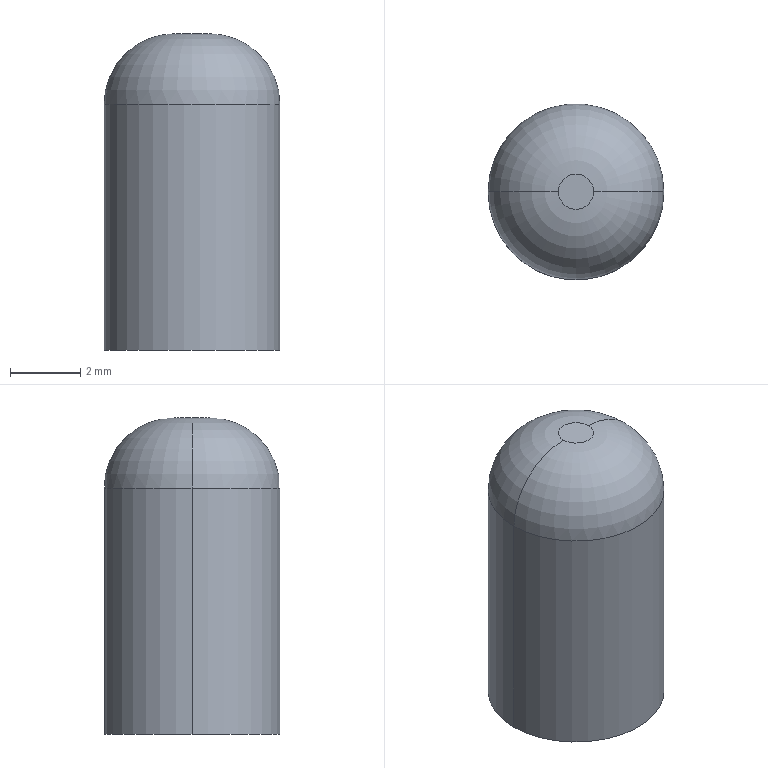Part | SolidWorks | features BaseBody 1 | 1 solid | 6 faces | box 5 x 5 x 9 mm | volume 165.64 mm3 | cylinder 2 | torus 2 | plane 2 | commonest cylinder face diameters 5 x2
STEP:
#1=CARTESIAN_POINT('',(6.125,1.871,0.));
#2=VERTEX_POINT('',#1);
#3=CARTESIAN_POINT('',(1.125,1.871,0.));
#4=VERTEX_POINT('',#3);
#5=CARTESIAN_POINT('',(3.625,1.871,0.));
#6=DIRECTION('',(0.,0.,1.));
#7=DIRECTION('',(1.,0.,0.));
#8=AXIS2_PLACEMENT_3D('',#5,#6,#7);
#9=CIRCLE('',#8,2.5);
#10=EDGE_CURVE('',#2,#4,#9,.T.);
#11=ORIENTED_EDGE('',*,*,#10,.T.);
#12=CARTESIAN_POINT('',(1.125,1.871,7.));
#13=VERTEX_POINT('',#12);
#14=CARTESIAN_POINT('',(1.125,1.871,0.));
#15=DIRECTION('',(0.,0.,1.));
#16=VECTOR('',#15,1000.);
#17=LINE('',#14,#16);
#18=EDGE_CURVE('',#4,#13,#17,.T.);
#19=ORIENTED_EDGE('',*,*,#18,.T.);
#20=CARTESIAN_POINT('',(6.125,1.871,7.));
#21=VERTEX_POINT('',#20);
#22=CARTESIAN_POINT('',(3.625,1.871,7.));
#23=DIRECTION('',(0.,0.,-1.));
#24=DIRECTION('',(1.,0.,0.));
#25=AXIS2_PLACEMENT_3D('',#22,#23,#24);
#26=CIRCLE('',#25,2.5);
#27=EDGE_CURVE('',#13,#21,#26,.T.);
#28=ORIENTED_EDGE('',*,*,#27,.T.);
#29=CARTESIAN_POINT('',(6.125,1.871,0.));
#30=DIRECTION('',(0.,0.,1.));
#31=VECTOR('',#30,1000.);
#32=LINE('',#29,#31);
#33=EDGE_CURVE('',#2,#21,#32,.T.);
#34=ORIENTED_EDGE('',*,*,#33,.F.);
#35=EDGE_LOOP('',(#11,#19,#28,#34));
#36=FACE_OUTER_BOUND('',#35,.T.);
#37=CARTESIAN_POINT('',(3.625,1.871,0.));
#38=DIRECTION('',(0.,0.,1.));
#39=DIRECTION('',(1.,0.,0.));
#40=AXIS2_PLACEMENT_3D('',#37,#38,#39);
#41=CYLINDRICAL_SURFACE('',#40,2.5);
#42=ADVANCED_FACE('',(#36),#41,.T.);
#43=ORIENTED_EDGE('',*,*,#27,.F.);
#44=CARTESIAN_POINT('',(3.125,1.871,9.));
#45=VERTEX_POINT('',#44);
#46=CARTESIAN_POINT('',(3.125,1.871,7.));
#47=DIRECTION('',(0.,1.,0.));
#48=DIRECTION('',(-1.,0.,0.));
#49=AXIS2_PLACEMENT_3D('',#46,#47,#48);
#50=CIRCLE('',#49,2.);
#51=EDGE_CURVE('',#13,#45,#50,.T.);
#52=ORIENTED_EDGE('',*,*,#51,.T.);
#53=CARTESIAN_POINT('',(4.125,1.871,9.));
#54=VERTEX_POINT('',#53);
#55=CARTESIAN_POINT('',(3.625,1.871,9.));
#56=DIRECTION('',(0.,0.,-1.));
#57=DIRECTION('',(1.,0.,0.));
#58=AXIS2_PLACEMENT_3D('',#55,#56,#57);
#59=CIRCLE('',#58,0.5);
#60=EDGE_CURVE('',#45,#54,#59,.T.);
#61=ORIENTED_EDGE('',*,*,#60,.T.);
#62=CARTESIAN_POINT('',(4.125,1.871,7.));
#63=DIRECTION('',(0.,-1.,0.));
#64=DIRECTION('',(0.,0.,-1.));
#65=AXIS2_PLACEMENT_3D('',#62,#63,#64);
#66=CIRCLE('',#65,2.);
#67=EDGE_CURVE('',#21,#54,#66,.T.);
#68=ORIENTED_EDGE('',*,*,#67,.F.);
#69=EDGE_LOOP('',(#43,#52,#61,#68));
#70=FACE_OUTER_BOUND('',#69,.T.);
#71=CARTESIAN_POINT('',(3.625,1.871,7.));
#72=DIRECTION('',(0.,0.,1.));
#73=DIRECTION('',(1.,0.,0.));
#74=AXIS2_PLACEMENT_3D('',#71,#72,#73);
#75=TOROIDAL_SURFACE('',#74,0.5,2.);
#76=ADVANCED_FACE('',(#70),#75,.T.);
#77=ORIENTED_EDGE('',*,*,#18,.F.);
#78=CARTESIAN_POINT('',(3.625,1.871,0.));
#79=DIRECTION('',(0.,0.,1.));
#80=DIRECTION('',(1.,0.,0.));
#81=AXIS2_PLACEMENT_3D('',#78,#79,#80);
#82=CIRCLE('',#81,2.5);
#83=EDGE_CURVE('',#4,#2,#82,.T.);
#84=ORIENTED_EDGE('',*,*,#83,.T.);
#85=ORIENTED_EDGE('',*,*,#33,.T.);
#86=CARTESIAN_POINT('',(3.625,1.871,7.));
#87=DIRECTION('',(0.,0.,-1.));
#88=DIRECTION('',(1.,0.,0.));
#89=AXIS2_PLACEMENT_3D('',#86,#87,#88);
#90=CIRCLE('',#89,2.5);
#91=EDGE_CURVE('',#21,#13,#90,.T.);
#92=ORIENTED_EDGE('',*,*,#91,.T.);
#93=EDGE_LOOP('',(#77,#84,#85,#92));
#94=FACE_OUTER_BOUND('',#93,.T.);
#95=CARTESIAN_POINT('',(3.625,1.871,0.));
#96=DIRECTION('',(0.,0.,1.));
#97=DIRECTION('',(1.,0.,0.));
#98=AXIS2_PLACEMENT_3D('',#95,#96,#97);
#99=CYLINDRICAL_SURFACE('',#98,2.5);
#100=ADVANCED_FACE('',(#94),#99,.T.);
#101=ORIENTED_EDGE('',*,*,#51,.F.);
#102=ORIENTED_EDGE('',*,*,#91,.F.);
#103=ORIENTED_EDGE('',*,*,#67,.T.);
#104=CARTESIAN_POINT('',(3.625,1.871,9.));
#105=DIRECTION('',(0.,0.,-1.));
#106=DIRECTION('',(1.,0.,0.));
#107=AXIS2_PLACEMENT_3D('',#104,#105,#106);
#108=CIRCLE('',#107,0.5);
#109=EDGE_CURVE('',#54,#45,#108,.T.);
#110=ORIENTED_EDGE('',*,*,#109,.T.);
#111=EDGE_LOOP('',(#101,#102,#103,#110));
#112=FACE_OUTER_BOUND('',#111,.T.);
#113=CARTESIAN_POINT('',(3.625,1.871,7.));
#114=DIRECTION('',(0.,0.,1.));
#115=DIRECTION('',(1.,0.,0.));
#116=AXIS2_PLACEMENT_3D('',#113,#114,#115);
#117=TOROIDAL_SURFACE('',#116,0.5,2.);
#118=ADVANCED_FACE('',(#112),#117,.T.);
#119=ORIENTED_EDGE('',*,*,#10,.F.);
#120=ORIENTED_EDGE('',*,*,#83,.F.);
#121=EDGE_LOOP('',(#119,#120));
#122=FACE_OUTER_BOUND('',#121,.T.);
#123=CARTESIAN_POINT('',(3.625,1.871,0.));
#124=DIRECTION('',(0.,0.,-1.));
#125=DIRECTION('',(-1.,0.,0.));
#126=AXIS2_PLACEMENT_3D('',#123,#124,#125);
#127=PLANE('',#126);
#128=ADVANCED_FACE('',(#122),#127,.T.);
#129=ORIENTED_EDGE('',*,*,#109,.F.);
#130=ORIENTED_EDGE('',*,*,#60,.F.);
#131=EDGE_LOOP('',(#129,#130));
#132=FACE_OUTER_BOUND('',#131,.T.);
#133=CARTESIAN_POINT('',(3.625,1.871,9.));
#134=DIRECTION('',(0.,0.,-1.));
#135=DIRECTION('',(-1.,0.,0.));
#136=AXIS2_PLACEMENT_3D('',#133,#134,#135);
#137=PLANE('',#136);
#138=ADVANCED_FACE('',(#132),#137,.F.);
#139=CLOSED_SHELL('',(#42,#76,#100,#118,#128,#138));
#140=MANIFOLD_SOLID_BREP('',#139);
#141=CARTESIAN_POINT('',(0.,0.,0.));
#142=DIRECTION('',(0.,0.,1.));
#143=DIRECTION('',(1.,0.,0.));
#144=AXIS2_PLACEMENT_3D('',#141,#142,#143);
#145=(LENGTH_UNIT()NAMED_UNIT(*)SI_UNIT(.MILLI.,.METRE.));
#146=UNCERTAINTY_MEASURE_WITH_UNIT(LENGTH_MEASURE(0.00001),#145,'','');
#147=(NAMED_UNIT(*)PLANE_ANGLE_UNIT()SI_UNIT($,.RADIAN.));
#148=(NAMED_UNIT(*)SI_UNIT($,.STERADIAN.)SOLID_ANGLE_UNIT());
#149=(GEOMETRIC_REPRESENTATION_CONTEXT(3)GLOBAL_UNCERTAINTY_ASSIGNED_CONTEXT((#146))GLOBAL_UNIT_ASSIGNED_CONTEXT((#145,#147,#148))REPRESENTATION_CONTEXT('',''));
#150=ADVANCED_BREP_SHAPE_REPRESENTATION('',(#140,#144),#149);